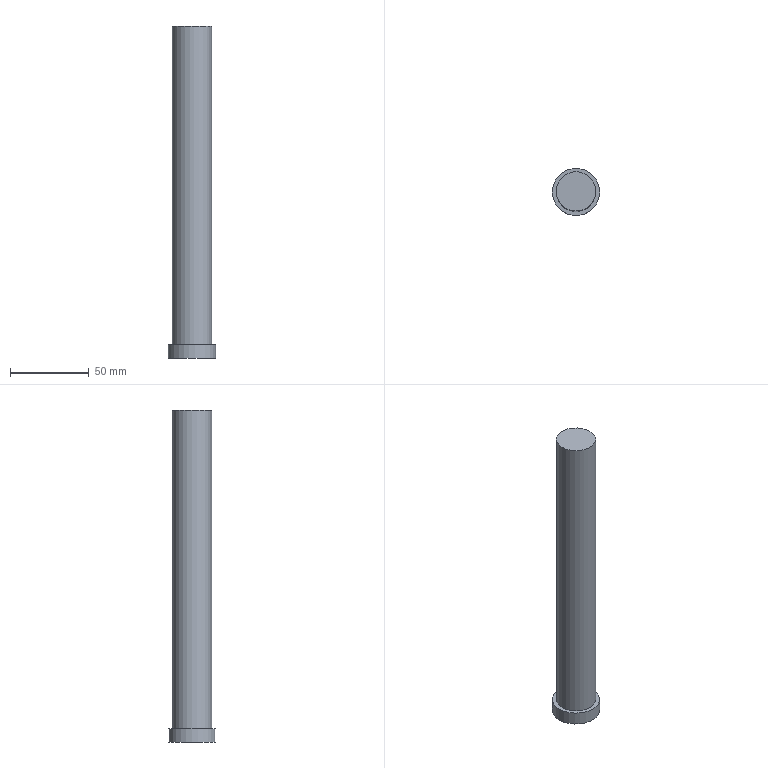Part | NX | features MPPJ 2 | 1 solid | 5 faces | box 30 x 30 x 211 mm | volume 105410 mm3 | plane 3 | cylinder 2 | commonest cylinder face diameters 25 x1 30 x1
STEP:
#1=CARTESIAN_POINT('',(94.5,-145.,0.5));
#2=VERTEX_POINT('',#1);
#3=CARTESIAN_POINT('',(82.,-145.,0.5));
#4=DIRECTION('',(0.,0.,-1.));
#5=DIRECTION('',(1.,0.,0.));
#6=AXIS2_PLACEMENT_3D('',#3,#4,#5);
#7=CIRCLE('',#6,12.5);
#8=EDGE_CURVE('',#2,#2,#7,.T.);
#9=ORIENTED_EDGE('',*,*,#8,.F.);
#10=EDGE_LOOP('',(#9));
#11=FACE_BOUND('',#10,.T.);
#12=CARTESIAN_POINT('',(82.,-145.,0.5));
#13=DIRECTION('',(0.,0.,1.));
#14=DIRECTION('',(1.,0.,0.));
#15=AXIS2_PLACEMENT_3D('',#12,#13,#14);
#16=PLANE('',#15);
#17=ADVANCED_FACE('',(#11),#16,.T.);
#18=CARTESIAN_POINT('',(94.5,-145.,-202.));
#19=VERTEX_POINT('',#18);
#20=CARTESIAN_POINT('',(82.,-145.,-202.));
#21=DIRECTION('',(0.,0.,1.));
#22=DIRECTION('',(1.,0.,0.));
#23=AXIS2_PLACEMENT_3D('',#20,#21,#22);
#24=CIRCLE('',#23,12.5);
#25=EDGE_CURVE('',#19,#19,#24,.F.);
#26=ORIENTED_EDGE('',*,*,#25,.F.);
#27=EDGE_LOOP('',(#26));
#28=FACE_BOUND('',#27,.T.);
#29=ORIENTED_EDGE('',*,*,#8,.T.);
#30=EDGE_LOOP('',(#29));
#31=FACE_BOUND('',#30,.T.);
#32=CARTESIAN_POINT('',(82.,-145.,-210.5));
#33=DIRECTION('',(0.,0.,1.));
#34=DIRECTION('',(1.,0.,0.));
#35=AXIS2_PLACEMENT_3D('',#32,#33,#34);
#36=CYLINDRICAL_SURFACE('',#35,12.5);
#37=ADVANCED_FACE('',(#28,#31),#36,.T.);
#38=ORIENTED_EDGE('',*,*,#25,.T.);
#39=EDGE_LOOP('',(#38));
#40=FACE_BOUND('',#39,.T.);
#41=CARTESIAN_POINT('',(97.,-145.,-202.));
#42=VERTEX_POINT('',#41);
#43=CARTESIAN_POINT('',(82.,-145.,-202.));
#44=DIRECTION('',(0.,0.,-1.));
#45=DIRECTION('',(1.,0.,0.));
#46=AXIS2_PLACEMENT_3D('',#43,#44,#45);
#47=CIRCLE('',#46,15.);
#48=EDGE_CURVE('',#42,#42,#47,.T.);
#49=ORIENTED_EDGE('',*,*,#48,.F.);
#50=EDGE_LOOP('',(#49));
#51=FACE_BOUND('',#50,.T.);
#52=CARTESIAN_POINT('',(82.,-145.,-202.));
#53=DIRECTION('',(0.,0.,1.));
#54=DIRECTION('',(1.,0.,0.));
#55=AXIS2_PLACEMENT_3D('',#52,#53,#54);
#56=PLANE('',#55);
#57=ADVANCED_FACE('',(#40,#51),#56,.T.);
#58=ORIENTED_EDGE('',*,*,#48,.T.);
#59=EDGE_LOOP('',(#58));
#60=FACE_BOUND('',#59,.T.);
#61=CARTESIAN_POINT('',(97.,-145.,-210.5));
#62=VERTEX_POINT('',#61);
#63=CARTESIAN_POINT('',(82.,-145.,-210.5));
#64=DIRECTION('',(0.,0.,1.));
#65=DIRECTION('',(1.,0.,0.));
#66=AXIS2_PLACEMENT_3D('',#63,#64,#65);
#67=CIRCLE('',#66,15.);
#68=EDGE_CURVE('',#62,#62,#67,.T.);
#69=ORIENTED_EDGE('',*,*,#68,.T.);
#70=EDGE_LOOP('',(#69));
#71=FACE_BOUND('',#70,.T.);
#72=CARTESIAN_POINT('',(82.,-145.,-210.5));
#73=DIRECTION('',(0.,0.,1.));
#74=DIRECTION('',(1.,0.,0.));
#75=AXIS2_PLACEMENT_3D('',#72,#73,#74);
#76=CYLINDRICAL_SURFACE('',#75,15.);
#77=ADVANCED_FACE('',(#60,#71),#76,.T.);
#78=ORIENTED_EDGE('',*,*,#68,.F.);
#79=EDGE_LOOP('',(#78));
#80=FACE_BOUND('',#79,.T.);
#81=CARTESIAN_POINT('',(82.,-145.,-210.5));
#82=DIRECTION('',(0.,0.,-1.));
#83=DIRECTION('',(-1.,0.,0.));
#84=AXIS2_PLACEMENT_3D('',#81,#82,#83);
#85=PLANE('',#84);
#86=ADVANCED_FACE('',(#80),#85,.T.);
#87=CLOSED_SHELL('',(#17,#37,#57,#77,#86));
#88=MANIFOLD_SOLID_BREP('',#87);
#89=(LENGTH_UNIT()NAMED_UNIT(*)SI_UNIT(.MILLI.,.METRE.));
#90=UNCERTAINTY_MEASURE_WITH_UNIT(LENGTH_MEASURE(0.00001),#89,'','');
#91=(NAMED_UNIT(*)PLANE_ANGLE_UNIT()SI_UNIT($,.RADIAN.));
#92=(NAMED_UNIT(*)SI_UNIT($,.STERADIAN.)SOLID_ANGLE_UNIT());
#93=(GEOMETRIC_REPRESENTATION_CONTEXT(3)GLOBAL_UNCERTAINTY_ASSIGNED_CONTEXT((#90))GLOBAL_UNIT_ASSIGNED_CONTEXT((#89,#91,#92))REPRESENTATION_CONTEXT('',''));
#94=ADVANCED_BREP_SHAPE_REPRESENTATION('',(#88),#93);